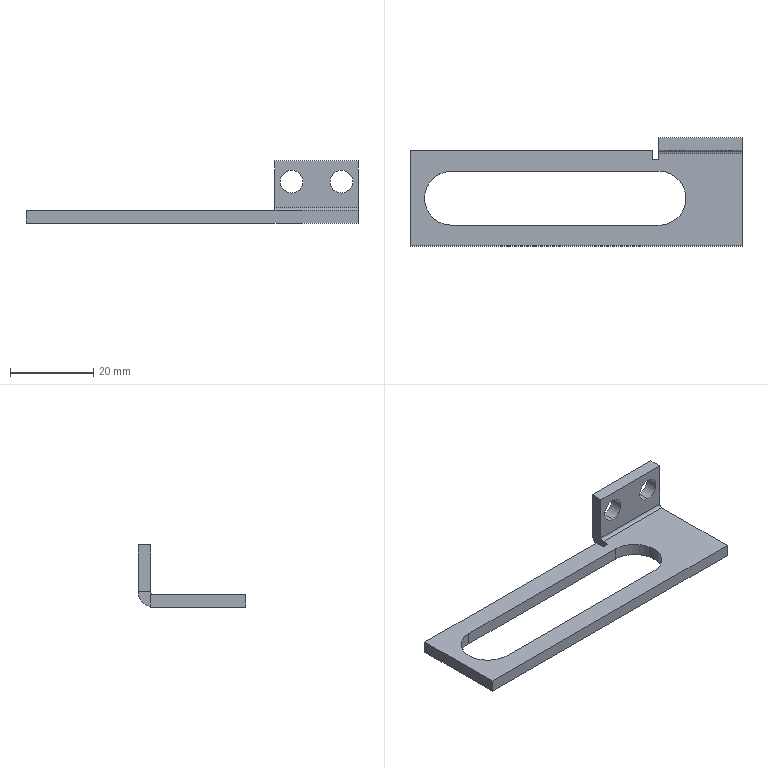Part | STEP file | detection sheet metal_default | 1 solid | 27 faces | box 80 x 26 x 15 mm | volume 3862 mm3 | plane 18 | cylinder 9 | commonest cylinder face diameters 5.5 x4 13 x3 1.473 x1 7.473 x1